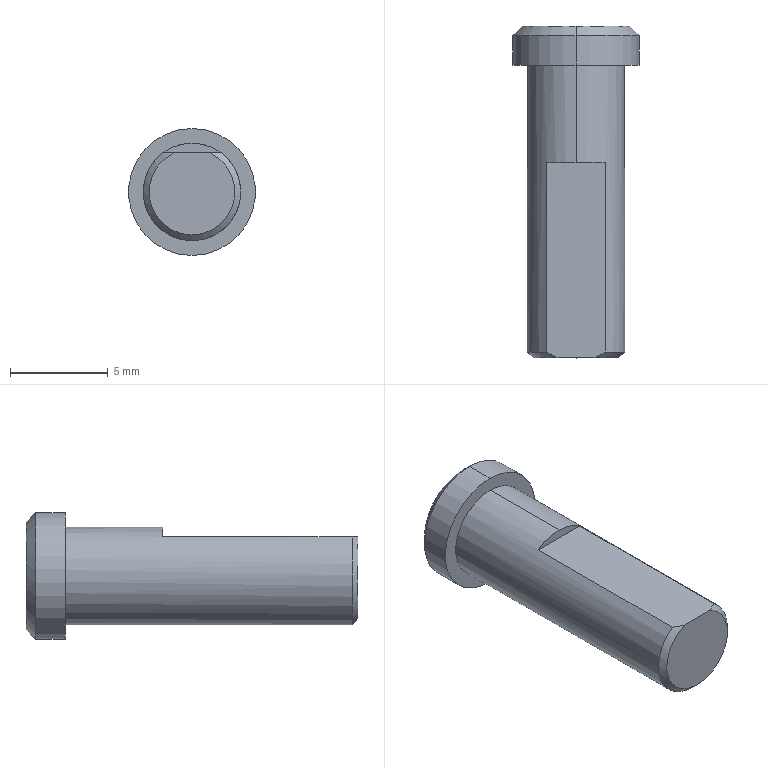Part | SolidWorks | features Chamfer 2, ICE 2, Extrusion 1 | 1 solid | 12 faces | box 6.5 x 17 x 6.5 mm | volume 347.697 mm3 | plane 5 | cylinder 4 | cone 3 | commonest cylinder face diameters 5 x2 6.5 x2
STEP:
#1=CARTESIAN_POINT('',(0.,17.,2.75));
#2=VERTEX_POINT('',#1);
#3=CARTESIAN_POINT('',(0.,17.,-2.75));
#4=VERTEX_POINT('',#3);
#5=CARTESIAN_POINT('',(0.,17.,0.));
#6=DIRECTION('',(0.,1.,0.));
#7=DIRECTION('',(0.,0.,1.));
#8=AXIS2_PLACEMENT_3D('',#5,#6,#7);
#9=CIRCLE('',#8,2.75);
#10=EDGE_CURVE('',#2,#4,#9,.T.);
#11=ORIENTED_EDGE('',*,*,#10,.F.);
#12=CARTESIAN_POINT('',(0.,16.5,3.25));
#13=VERTEX_POINT('',#12);
#14=CARTESIAN_POINT('',(0.,17.,2.75));
#15=DIRECTION('',(0.,-0.7071,0.7071));
#16=VECTOR('',#15,1000.);
#17=LINE('',#14,#16);
#18=EDGE_CURVE('',#2,#13,#17,.T.);
#19=ORIENTED_EDGE('',*,*,#18,.T.);
#20=CARTESIAN_POINT('',(0.,16.5,-3.25));
#21=VERTEX_POINT('',#20);
#22=CARTESIAN_POINT('',(0.,16.5,0.));
#23=DIRECTION('',(0.,-1.,0.));
#24=DIRECTION('',(0.,0.,1.));
#25=AXIS2_PLACEMENT_3D('',#22,#23,#24);
#26=CIRCLE('',#25,3.25);
#27=EDGE_CURVE('',#21,#13,#26,.T.);
#28=ORIENTED_EDGE('',*,*,#27,.F.);
#29=CARTESIAN_POINT('',(0.,17.,-2.75));
#30=DIRECTION('',(0.,-0.7071,-0.7071));
#31=VECTOR('',#30,1000.);
#32=LINE('',#29,#31);
#33=EDGE_CURVE('',#4,#21,#32,.T.);
#34=ORIENTED_EDGE('',*,*,#33,.F.);
#35=EDGE_LOOP('',(#11,#19,#28,#34));
#36=FACE_OUTER_BOUND('',#35,.T.);
#37=CARTESIAN_POINT('',(0.,17.,0.));
#38=DIRECTION('',(0.,-1.,0.));
#39=DIRECTION('',(0.,0.,-1.));
#40=AXIS2_PLACEMENT_3D('',#37,#38,#39);
#41=CONICAL_SURFACE('',#40,2.75,0.7854);
#42=ADVANCED_FACE('',(#36),#41,.T.);
#43=ORIENTED_EDGE('',*,*,#27,.T.);
#44=CARTESIAN_POINT('',(0.,15.,3.25));
#45=VERTEX_POINT('',#44);
#46=CARTESIAN_POINT('',(0.,17.,3.25));
#47=DIRECTION('',(0.,-1.,0.));
#48=VECTOR('',#47,1000.);
#49=LINE('',#46,#48);
#50=EDGE_CURVE('',#13,#45,#49,.T.);
#51=ORIENTED_EDGE('',*,*,#50,.T.);
#52=CARTESIAN_POINT('',(0.,15.,-3.25));
#53=VERTEX_POINT('',#52);
#54=CARTESIAN_POINT('',(0.,15.,0.));
#55=DIRECTION('',(0.,1.,0.));
#56=DIRECTION('',(0.,0.,1.));
#57=AXIS2_PLACEMENT_3D('',#54,#55,#56);
#58=CIRCLE('',#57,3.25);
#59=EDGE_CURVE('',#45,#53,#58,.T.);
#60=ORIENTED_EDGE('',*,*,#59,.T.);
#61=CARTESIAN_POINT('',(0.,17.,-3.25));
#62=DIRECTION('',(0.,-1.,0.));
#63=VECTOR('',#62,1000.);
#64=LINE('',#61,#63);
#65=EDGE_CURVE('',#21,#53,#64,.T.);
#66=ORIENTED_EDGE('',*,*,#65,.F.);
#67=EDGE_LOOP('',(#43,#51,#60,#66));
#68=FACE_OUTER_BOUND('',#67,.T.);
#69=CARTESIAN_POINT('',(0.,17.,0.));
#70=DIRECTION('',(0.,-1.,0.));
#71=DIRECTION('',(0.,0.,-1.));
#72=AXIS2_PLACEMENT_3D('',#69,#70,#71);
#73=CYLINDRICAL_SURFACE('',#72,3.25);
#74=ADVANCED_FACE('',(#68),#73,.T.);
#75=CARTESIAN_POINT('',(0.,15.,2.5));
#76=VERTEX_POINT('',#75);
#77=CARTESIAN_POINT('',(0.,15.,-2.5));
#78=VERTEX_POINT('',#77);
#79=CARTESIAN_POINT('',(0.,15.,0.));
#80=DIRECTION('',(0.,1.,0.));
#81=DIRECTION('',(0.,0.,1.));
#82=AXIS2_PLACEMENT_3D('',#79,#80,#81);
#83=CIRCLE('',#82,2.5);
#84=EDGE_CURVE('',#76,#78,#83,.T.);
#85=ORIENTED_EDGE('',*,*,#84,.F.);
#86=CARTESIAN_POINT('',(0.,10.,2.5));
#87=VERTEX_POINT('',#86);
#88=CARTESIAN_POINT('',(0.,15.,2.5));
#89=DIRECTION('',(0.,-1.,0.));
#90=VECTOR('',#89,1000.);
#91=LINE('',#88,#90);
#92=EDGE_CURVE('',#76,#87,#91,.T.);
#93=ORIENTED_EDGE('',*,*,#92,.T.);
#94=CARTESIAN_POINT('',(1.5,10.,2.));
#95=VERTEX_POINT('',#94);
#96=CARTESIAN_POINT('',(0.,10.,0.));
#97=DIRECTION('',(0.,-1.,0.));
#98=DIRECTION('',(0.,0.,-1.));
#99=AXIS2_PLACEMENT_3D('',#96,#97,#98);
#100=CIRCLE('',#99,2.5);
#101=EDGE_CURVE('',#95,#87,#100,.T.);
#102=ORIENTED_EDGE('',*,*,#101,.F.);
#103=CARTESIAN_POINT('',(1.5,0.3,2.));
#104=VERTEX_POINT('',#103);
#105=CARTESIAN_POINT('',(1.5,15.,2.));
#106=DIRECTION('',(0.,-1.,0.));
#107=VECTOR('',#106,1000.);
#108=LINE('',#105,#107);
#109=EDGE_CURVE('',#95,#104,#108,.T.);
#110=ORIENTED_EDGE('',*,*,#109,.T.);
#111=CARTESIAN_POINT('',(0.,0.3,-2.5));
#112=VERTEX_POINT('',#111);
#113=CARTESIAN_POINT('',(0.,0.3,0.));
#114=DIRECTION('',(0.,1.,0.));
#115=DIRECTION('',(0.,0.,1.));
#116=AXIS2_PLACEMENT_3D('',#113,#114,#115);
#117=CIRCLE('',#116,2.5);
#118=EDGE_CURVE('',#104,#112,#117,.T.);
#119=ORIENTED_EDGE('',*,*,#118,.T.);
#120=CARTESIAN_POINT('',(0.,15.,-2.5));
#121=DIRECTION('',(0.,-1.,0.));
#122=VECTOR('',#121,1000.);
#123=LINE('',#120,#122);
#124=EDGE_CURVE('',#78,#112,#123,.T.);
#125=ORIENTED_EDGE('',*,*,#124,.F.);
#126=EDGE_LOOP('',(#85,#93,#102,#110,#119,#125));
#127=FACE_OUTER_BOUND('',#126,.T.);
#128=CARTESIAN_POINT('',(0.,15.,0.));
#129=DIRECTION('',(0.,-1.,0.));
#130=DIRECTION('',(0.,0.,-1.));
#131=AXIS2_PLACEMENT_3D('',#128,#129,#130);
#132=CYLINDRICAL_SURFACE('',#131,2.5);
#133=ADVANCED_FACE('',(#127),#132,.T.);
#134=ORIENTED_EDGE('',*,*,#92,.F.);
#135=CARTESIAN_POINT('',(0.,15.,0.));
#136=DIRECTION('',(0.,1.,0.));
#137=DIRECTION('',(0.,0.,1.));
#138=AXIS2_PLACEMENT_3D('',#135,#136,#137);
#139=CIRCLE('',#138,2.5);
#140=EDGE_CURVE('',#78,#76,#139,.T.);
#141=ORIENTED_EDGE('',*,*,#140,.F.);
#142=ORIENTED_EDGE('',*,*,#124,.T.);
#143=CARTESIAN_POINT('',(-1.5,0.3,2.));
#144=VERTEX_POINT('',#143);
#145=CARTESIAN_POINT('',(0.,0.3,0.));
#146=DIRECTION('',(0.,1.,0.));
#147=DIRECTION('',(0.,0.,1.));
#148=AXIS2_PLACEMENT_3D('',#145,#146,#147);
#149=CIRCLE('',#148,2.5);
#150=EDGE_CURVE('',#112,#144,#149,.T.);
#151=ORIENTED_EDGE('',*,*,#150,.T.);
#152=CARTESIAN_POINT('',(-1.5,10.,2.));
#153=VERTEX_POINT('',#152);
#154=CARTESIAN_POINT('',(-1.5,15.,2.));
#155=DIRECTION('',(0.,1.,0.));
#156=VECTOR('',#155,1000.);
#157=LINE('',#154,#156);
#158=EDGE_CURVE('',#144,#153,#157,.T.);
#159=ORIENTED_EDGE('',*,*,#158,.T.);
#160=CARTESIAN_POINT('',(0.,10.,0.));
#161=DIRECTION('',(0.,-1.,0.));
#162=DIRECTION('',(0.,0.,-1.));
#163=AXIS2_PLACEMENT_3D('',#160,#161,#162);
#164=CIRCLE('',#163,2.5);
#165=EDGE_CURVE('',#87,#153,#164,.T.);
#166=ORIENTED_EDGE('',*,*,#165,.F.);
#167=EDGE_LOOP('',(#134,#141,#142,#151,#159,#166));
#168=FACE_OUTER_BOUND('',#167,.T.);
#169=CARTESIAN_POINT('',(0.,15.,0.));
#170=DIRECTION('',(0.,-1.,0.));
#171=DIRECTION('',(0.,0.,-1.));
#172=AXIS2_PLACEMENT_3D('',#169,#170,#171);
#173=CYLINDRICAL_SURFACE('',#172,2.5);
#174=ADVANCED_FACE('',(#168),#173,.T.);
#175=CARTESIAN_POINT('',(-0.9165,0.,2.));
#176=VERTEX_POINT('',#175);
#177=CARTESIAN_POINT('',(0.9165,0.,2.));
#178=VERTEX_POINT('',#177);
#179=CARTESIAN_POINT('',(0.,0.,0.));
#180=DIRECTION('',(0.,-1.,0.));
#181=DIRECTION('',(0.,0.,1.));
#182=AXIS2_PLACEMENT_3D('',#179,#180,#181);
#183=CIRCLE('',#182,2.2);
#184=EDGE_CURVE('',#176,#178,#183,.T.);
#185=ORIENTED_EDGE('',*,*,#184,.T.);
#186=CARTESIAN_POINT('',(-2.957,0.,2.));
#187=DIRECTION('',(1.,0.,0.));
#188=VECTOR('',#187,1000.);
#189=LINE('',#186,#188);
#190=EDGE_CURVE('',#176,#178,#189,.T.);
#191=ORIENTED_EDGE('',*,*,#190,.F.);
#192=EDGE_LOOP('',(#185,#191));
#193=FACE_OUTER_BOUND('',#192,.T.);
#194=CARTESIAN_POINT('',(0.,0.,0.));
#195=DIRECTION('',(0.,1.,0.));
#196=DIRECTION('',(0.,0.,1.));
#197=AXIS2_PLACEMENT_3D('',#194,#195,#196);
#198=PLANE('',#197);
#199=ADVANCED_FACE('',(#193),#198,.F.);
#200=CARTESIAN_POINT('',(0.,15.,0.));
#201=DIRECTION('',(0.,1.,0.));
#202=DIRECTION('',(0.,0.,1.));
#203=AXIS2_PLACEMENT_3D('',#200,#201,#202);
#204=CIRCLE('',#203,3.25);
#205=EDGE_CURVE('',#53,#45,#204,.T.);
#206=ORIENTED_EDGE('',*,*,#205,.F.);
#207=ORIENTED_EDGE('',*,*,#59,.F.);
#208=EDGE_LOOP('',(#206,#207));
#209=FACE_OUTER_BOUND('',#208,.T.);
#210=ORIENTED_EDGE('',*,*,#140,.T.);
#211=ORIENTED_EDGE('',*,*,#84,.T.);
#212=EDGE_LOOP('',(#210,#211));
#213=FACE_BOUND('',#212,.T.);
#214=CARTESIAN_POINT('',(0.,15.,0.));
#215=DIRECTION('',(0.,1.,0.));
#216=DIRECTION('',(0.,0.,1.));
#217=AXIS2_PLACEMENT_3D('',#214,#215,#216);
#218=PLANE('',#217);
#219=ADVANCED_FACE('',(#209,#213),#218,.F.);
#220=ORIENTED_EDGE('',*,*,#50,.F.);
#221=CARTESIAN_POINT('',(0.,16.5,0.));
#222=DIRECTION('',(0.,-1.,0.));
#223=DIRECTION('',(0.,0.,1.));
#224=AXIS2_PLACEMENT_3D('',#221,#222,#223);
#225=CIRCLE('',#224,3.25);
#226=EDGE_CURVE('',#13,#21,#225,.T.);
#227=ORIENTED_EDGE('',*,*,#226,.T.);
#228=ORIENTED_EDGE('',*,*,#65,.T.);
#229=ORIENTED_EDGE('',*,*,#205,.T.);
#230=EDGE_LOOP('',(#220,#227,#228,#229));
#231=FACE_OUTER_BOUND('',#230,.T.);
#232=CARTESIAN_POINT('',(0.,17.,0.));
#233=DIRECTION('',(0.,-1.,0.));
#234=DIRECTION('',(0.,0.,-1.));
#235=AXIS2_PLACEMENT_3D('',#232,#233,#234);
#236=CYLINDRICAL_SURFACE('',#235,3.25);
#237=ADVANCED_FACE('',(#231),#236,.T.);
#238=CARTESIAN_POINT('',(0.,17.,0.));
#239=DIRECTION('',(0.,1.,0.));
#240=DIRECTION('',(0.,0.,1.));
#241=AXIS2_PLACEMENT_3D('',#238,#239,#240);
#242=CIRCLE('',#241,2.75);
#243=EDGE_CURVE('',#4,#2,#242,.T.);
#244=ORIENTED_EDGE('',*,*,#243,.T.);
#245=ORIENTED_EDGE('',*,*,#10,.T.);
#246=EDGE_LOOP('',(#244,#245));
#247=FACE_OUTER_BOUND('',#246,.T.);
#248=CARTESIAN_POINT('',(0.,17.,0.));
#249=DIRECTION('',(0.,1.,0.));
#250=DIRECTION('',(0.,0.,1.));
#251=AXIS2_PLACEMENT_3D('',#248,#249,#250);
#252=PLANE('',#251);
#253=ADVANCED_FACE('',(#247),#252,.T.);
#254=ORIENTED_EDGE('',*,*,#18,.F.);
#255=ORIENTED_EDGE('',*,*,#243,.F.);
#256=ORIENTED_EDGE('',*,*,#33,.T.);
#257=ORIENTED_EDGE('',*,*,#226,.F.);
#258=EDGE_LOOP('',(#254,#255,#256,#257));
#259=FACE_OUTER_BOUND('',#258,.T.);
#260=CARTESIAN_POINT('',(0.,17.,0.));
#261=DIRECTION('',(0.,-1.,0.));
#262=DIRECTION('',(0.,0.,-1.));
#263=AXIS2_PLACEMENT_3D('',#260,#261,#262);
#264=CONICAL_SURFACE('',#263,2.75,0.7854);
#265=ADVANCED_FACE('',(#259),#264,.T.);
#266=CARTESIAN_POINT('',(-1.5,0.3,2.));
#267=CARTESIAN_POINT('',(-1.312,0.1871,2.));
#268=CARTESIAN_POINT('',(-1.119,0.08424,2.));
#269=CARTESIAN_POINT('',(-0.9165,0.,2.));
#270=B_SPLINE_CURVE_WITH_KNOTS('',3,(#266,#267,#268,#269),.UNSPECIFIED.,.F.,.F.,(4,4),(0.00472,0.005377),.UNSPECIFIED.);
#271=EDGE_CURVE('',#144,#176,#270,.T.);
#272=ORIENTED_EDGE('',*,*,#271,.F.);
#273=ORIENTED_EDGE('',*,*,#150,.F.);
#274=ORIENTED_EDGE('',*,*,#118,.F.);
#275=CARTESIAN_POINT('',(0.9165,0.,2.));
#276=CARTESIAN_POINT('',(1.12,0.08466,2.));
#277=CARTESIAN_POINT('',(1.313,0.1875,2.));
#278=CARTESIAN_POINT('',(1.5,0.3,2.));
#279=B_SPLINE_CURVE_WITH_KNOTS('',3,(#275,#276,#277,#278),.UNSPECIFIED.,.F.,.F.,(4,4),(0.007265,0.007928),.UNSPECIFIED.);
#280=EDGE_CURVE('',#178,#104,#279,.T.);
#281=ORIENTED_EDGE('',*,*,#280,.F.);
#282=ORIENTED_EDGE('',*,*,#184,.F.);
#283=EDGE_LOOP('',(#272,#273,#274,#281,#282));
#284=FACE_OUTER_BOUND('',#283,.T.);
#285=CARTESIAN_POINT('',(0.,0.3,0.));
#286=DIRECTION('',(0.,1.,0.));
#287=DIRECTION('',(0.,0.,1.));
#288=AXIS2_PLACEMENT_3D('',#285,#286,#287);
#289=CONICAL_SURFACE('',#288,2.5,0.7854);
#290=ADVANCED_FACE('',(#284),#289,.T.);
#291=ORIENTED_EDGE('',*,*,#101,.T.);
#292=ORIENTED_EDGE('',*,*,#165,.T.);
#293=CARTESIAN_POINT('',(-2.957,10.,2.));
#294=DIRECTION('',(1.,0.,0.));
#295=VECTOR('',#294,1000.);
#296=LINE('',#293,#295);
#297=EDGE_CURVE('',#153,#95,#296,.T.);
#298=ORIENTED_EDGE('',*,*,#297,.T.);
#299=EDGE_LOOP('',(#291,#292,#298));
#300=FACE_OUTER_BOUND('',#299,.T.);
#301=CARTESIAN_POINT('',(0.,10.,0.));
#302=DIRECTION('',(0.,-1.,0.));
#303=DIRECTION('',(0.,0.,-1.));
#304=AXIS2_PLACEMENT_3D('',#301,#302,#303);
#305=PLANE('',#304);
#306=ADVANCED_FACE('',(#300),#305,.T.);
#307=ORIENTED_EDGE('',*,*,#271,.T.);
#308=ORIENTED_EDGE('',*,*,#190,.T.);
#309=ORIENTED_EDGE('',*,*,#280,.T.);
#310=ORIENTED_EDGE('',*,*,#109,.F.);
#311=ORIENTED_EDGE('',*,*,#297,.F.);
#312=ORIENTED_EDGE('',*,*,#158,.F.);
#313=EDGE_LOOP('',(#307,#308,#309,#310,#311,#312));
#314=FACE_OUTER_BOUND('',#313,.T.);
#315=CARTESIAN_POINT('',(-2.957,10.,2.));
#316=DIRECTION('',(0.,0.,-1.));
#317=DIRECTION('',(-1.,0.,0.));
#318=AXIS2_PLACEMENT_3D('',#315,#316,#317);
#319=PLANE('',#318);
#320=ADVANCED_FACE('',(#314),#319,.F.);
#321=CLOSED_SHELL('',(#42,#74,#133,#174,#199,#219,#237,#253,#265,#290,#306,#320));
#322=MANIFOLD_SOLID_BREP('',#321);
#323=CARTESIAN_POINT('',(0.,0.,0.));
#324=DIRECTION('',(0.,0.,1.));
#325=DIRECTION('',(1.,0.,0.));
#326=AXIS2_PLACEMENT_3D('',#323,#324,#325);
#327=(LENGTH_UNIT()NAMED_UNIT(*)SI_UNIT(.MILLI.,.METRE.));
#328=UNCERTAINTY_MEASURE_WITH_UNIT(LENGTH_MEASURE(0.00001),#327,'','');
#329=(NAMED_UNIT(*)PLANE_ANGLE_UNIT()SI_UNIT($,.RADIAN.));
#330=(NAMED_UNIT(*)SI_UNIT($,.STERADIAN.)SOLID_ANGLE_UNIT());
#331=(GEOMETRIC_REPRESENTATION_CONTEXT(3)GLOBAL_UNCERTAINTY_ASSIGNED_CONTEXT((#328))GLOBAL_UNIT_ASSIGNED_CONTEXT((#327,#329,#330))REPRESENTATION_CONTEXT('',''));
#332=ADVANCED_BREP_SHAPE_REPRESENTATION('',(#322,#326),#331);